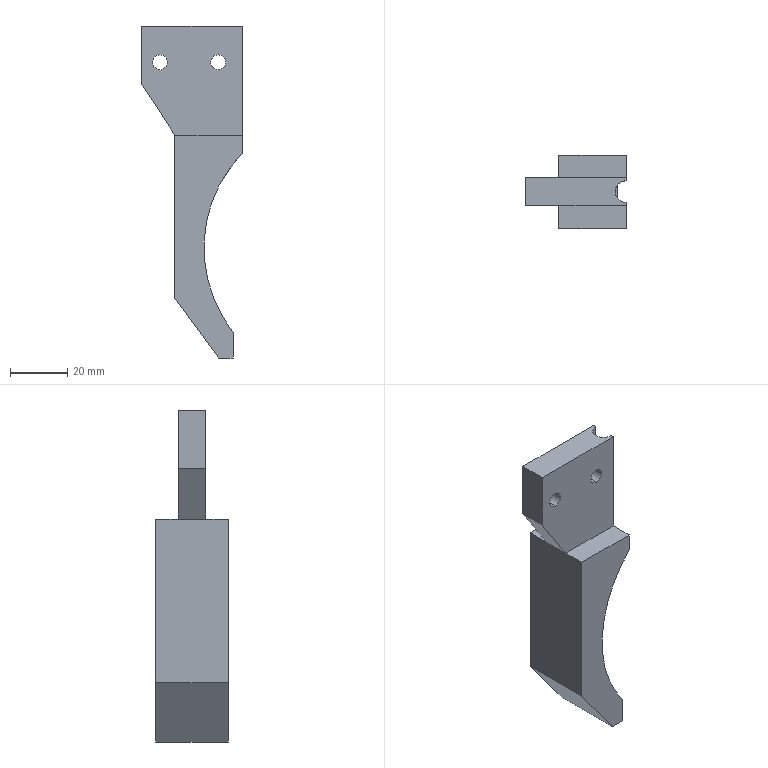Part | SolidWorks | features ICE 2, Extrusion 1 | 1 solid | 21 faces | box 35.052 x 25.4 x 115.945 mm | volume 36905 mm3 | plane 15 | cylinder 6 | commonest cylinder face diameters 5.207 x4 7.62 x1 95.25 x1
STEP:
#1=CARTESIAN_POINT('',(-8.382,4.826,62.197));
#2=VERTEX_POINT('',#1);
#3=CARTESIAN_POINT('',(-8.382,4.826,67.404));
#4=VERTEX_POINT('',#3);
#5=CARTESIAN_POINT('',(-8.382,4.826,64.801));
#6=DIRECTION('',(0.,1.,0.));
#7=DIRECTION('',(0.,0.,1.));
#8=AXIS2_PLACEMENT_3D('',#5,#6,#7);
#9=CIRCLE('',#8,2.603);
#10=EDGE_CURVE('',#2,#4,#9,.T.);
#11=ORIENTED_EDGE('',*,*,#10,.T.);
#12=CARTESIAN_POINT('',(-8.382,-4.826,67.404));
#13=VERTEX_POINT('',#12);
#14=CARTESIAN_POINT('',(-8.382,4.826,67.404));
#15=DIRECTION('',(0.,-1.,0.));
#16=VECTOR('',#15,1000.);
#17=LINE('',#14,#16);
#18=EDGE_CURVE('',#4,#13,#17,.T.);
#19=ORIENTED_EDGE('',*,*,#18,.T.);
#20=CARTESIAN_POINT('',(-8.382,-4.826,62.197));
#21=VERTEX_POINT('',#20);
#22=CARTESIAN_POINT('',(-8.382,-4.826,64.801));
#23=DIRECTION('',(0.,1.,0.));
#24=DIRECTION('',(0.,0.,1.));
#25=AXIS2_PLACEMENT_3D('',#22,#23,#24);
#26=CIRCLE('',#25,2.603);
#27=EDGE_CURVE('',#21,#13,#26,.T.);
#28=ORIENTED_EDGE('',*,*,#27,.F.);
#29=CARTESIAN_POINT('',(-8.382,4.826,62.197));
#30=DIRECTION('',(0.,-1.,0.));
#31=VECTOR('',#30,1000.);
#32=LINE('',#29,#31);
#33=EDGE_CURVE('',#2,#21,#32,.T.);
#34=ORIENTED_EDGE('',*,*,#33,.F.);
#35=EDGE_LOOP('',(#11,#19,#28,#34));
#36=FACE_OUTER_BOUND('',#35,.T.);
#37=CARTESIAN_POINT('',(-8.382,4.826,64.801));
#38=DIRECTION('',(0.,-1.,0.));
#39=DIRECTION('',(0.,0.,-1.));
#40=AXIS2_PLACEMENT_3D('',#37,#38,#39);
#41=CYLINDRICAL_SURFACE('',#40,2.603);
#42=ADVANCED_FACE('',(#36),#41,.F.);
#43=CARTESIAN_POINT('',(-28.702,4.826,62.197));
#44=VERTEX_POINT('',#43);
#45=CARTESIAN_POINT('',(-28.702,4.826,67.404));
#46=VERTEX_POINT('',#45);
#47=CARTESIAN_POINT('',(-28.702,4.826,64.801));
#48=DIRECTION('',(0.,1.,0.));
#49=DIRECTION('',(0.,0.,1.));
#50=AXIS2_PLACEMENT_3D('',#47,#48,#49);
#51=CIRCLE('',#50,2.603);
#52=EDGE_CURVE('',#44,#46,#51,.T.);
#53=ORIENTED_EDGE('',*,*,#52,.T.);
#54=CARTESIAN_POINT('',(-28.702,-4.826,67.404));
#55=VERTEX_POINT('',#54);
#56=CARTESIAN_POINT('',(-28.702,4.826,67.404));
#57=DIRECTION('',(0.,-1.,0.));
#58=VECTOR('',#57,1000.);
#59=LINE('',#56,#58);
#60=EDGE_CURVE('',#46,#55,#59,.T.);
#61=ORIENTED_EDGE('',*,*,#60,.T.);
#62=CARTESIAN_POINT('',(-28.702,-4.826,62.197));
#63=VERTEX_POINT('',#62);
#64=CARTESIAN_POINT('',(-28.702,-4.826,64.801));
#65=DIRECTION('',(0.,1.,0.));
#66=DIRECTION('',(0.,0.,1.));
#67=AXIS2_PLACEMENT_3D('',#64,#65,#66);
#68=CIRCLE('',#67,2.603);
#69=EDGE_CURVE('',#63,#55,#68,.T.);
#70=ORIENTED_EDGE('',*,*,#69,.F.);
#71=CARTESIAN_POINT('',(-28.702,4.826,62.197));
#72=DIRECTION('',(0.,-1.,0.));
#73=VECTOR('',#72,1000.);
#74=LINE('',#71,#73);
#75=EDGE_CURVE('',#44,#63,#74,.T.);
#76=ORIENTED_EDGE('',*,*,#75,.F.);
#77=EDGE_LOOP('',(#53,#61,#70,#76));
#78=FACE_OUTER_BOUND('',#77,.T.);
#79=CARTESIAN_POINT('',(-28.702,4.826,64.801));
#80=DIRECTION('',(0.,-1.,0.));
#81=DIRECTION('',(0.,0.,-1.));
#82=AXIS2_PLACEMENT_3D('',#79,#80,#81);
#83=CYLINDRICAL_SURFACE('',#82,2.604);
#84=ADVANCED_FACE('',(#78),#83,.F.);
#85=CARTESIAN_POINT('',(0.,3.81,33.051));
#86=VERTEX_POINT('',#85);
#87=CARTESIAN_POINT('',(0.,3.81,77.501));
#88=VERTEX_POINT('',#87);
#89=CARTESIAN_POINT('',(0.,3.81,27.463));
#90=DIRECTION('',(0.,0.,1.));
#91=VECTOR('',#90,1000.);
#92=LINE('',#89,#91);
#93=EDGE_CURVE('',#86,#88,#92,.T.);
#94=ORIENTED_EDGE('',*,*,#93,.F.);
#95=CARTESIAN_POINT('',(0.,12.7,33.051));
#96=VERTEX_POINT('',#95);
#97=CARTESIAN_POINT('',(0.,12.7,33.051));
#98=DIRECTION('',(0.,-1.,0.));
#99=VECTOR('',#98,1000.);
#100=LINE('',#97,#99);
#101=EDGE_CURVE('',#96,#86,#100,.T.);
#102=ORIENTED_EDGE('',*,*,#101,.F.);
#103=CARTESIAN_POINT('',(0.,12.7,39.401));
#104=VERTEX_POINT('',#103);
#105=CARTESIAN_POINT('',(0.,12.7,0.));
#106=DIRECTION('',(0.,0.,1.));
#107=VECTOR('',#106,1000.);
#108=LINE('',#105,#107);
#109=EDGE_CURVE('',#96,#104,#108,.T.);
#110=ORIENTED_EDGE('',*,*,#109,.T.);
#111=CARTESIAN_POINT('',(0.,4.826,39.401));
#112=VERTEX_POINT('',#111);
#113=CARTESIAN_POINT('',(0.,12.7,39.401));
#114=DIRECTION('',(0.,-1.,0.));
#115=VECTOR('',#114,1000.);
#116=LINE('',#113,#115);
#117=EDGE_CURVE('',#104,#112,#116,.T.);
#118=ORIENTED_EDGE('',*,*,#117,.T.);
#119=CARTESIAN_POINT('',(0.,4.826,77.501));
#120=VERTEX_POINT('',#119);
#121=CARTESIAN_POINT('',(0.,4.826,0.));
#122=DIRECTION('',(0.,0.,-1.));
#123=VECTOR('',#122,1000.);
#124=LINE('',#121,#123);
#125=EDGE_CURVE('',#120,#112,#124,.T.);
#126=ORIENTED_EDGE('',*,*,#125,.F.);
#127=CARTESIAN_POINT('',(0.,4.826,77.501));
#128=DIRECTION('',(0.,-1.,0.));
#129=VECTOR('',#128,1000.);
#130=LINE('',#127,#129);
#131=EDGE_CURVE('',#120,#88,#130,.T.);
#132=ORIENTED_EDGE('',*,*,#131,.T.);
#133=EDGE_LOOP('',(#94,#102,#110,#118,#126,#132));
#134=FACE_OUTER_BOUND('',#133,.T.);
#135=CARTESIAN_POINT('',(0.,12.7,0.));
#136=DIRECTION('',(1.,0.,0.));
#137=DIRECTION('',(0.,0.,-1.));
#138=AXIS2_PLACEMENT_3D('',#135,#136,#137);
#139=PLANE('',#138);
#140=ADVANCED_FACE('',(#134),#139,.T.);
#141=CARTESIAN_POINT('',(0.,-4.826,39.401));
#142=VERTEX_POINT('',#141);
#143=CARTESIAN_POINT('',(0.,-12.7,39.401));
#144=VERTEX_POINT('',#143);
#145=CARTESIAN_POINT('',(0.,12.7,39.401));
#146=DIRECTION('',(0.,-1.,0.));
#147=VECTOR('',#146,1000.);
#148=LINE('',#145,#147);
#149=EDGE_CURVE('',#142,#144,#148,.T.);
#150=ORIENTED_EDGE('',*,*,#149,.F.);
#151=CARTESIAN_POINT('',(-23.495,-4.826,39.401));
#152=VERTEX_POINT('',#151);
#153=CARTESIAN_POINT('',(0.,-4.826,39.401));
#154=DIRECTION('',(-1.,0.,0.));
#155=VECTOR('',#154,1000.);
#156=LINE('',#153,#155);
#157=EDGE_CURVE('',#142,#152,#156,.T.);
#158=ORIENTED_EDGE('',*,*,#157,.T.);
#159=CARTESIAN_POINT('',(-23.495,-12.7,39.401));
#160=VERTEX_POINT('',#159);
#161=CARTESIAN_POINT('',(-23.495,12.7,39.401));
#162=DIRECTION('',(0.,-1.,0.));
#163=VECTOR('',#162,1000.);
#164=LINE('',#161,#163);
#165=EDGE_CURVE('',#152,#160,#164,.T.);
#166=ORIENTED_EDGE('',*,*,#165,.T.);
#167=CARTESIAN_POINT('',(0.,-12.7,39.401));
#168=DIRECTION('',(-1.,0.,0.));
#169=VECTOR('',#168,1000.);
#170=LINE('',#167,#169);
#171=EDGE_CURVE('',#144,#160,#170,.T.);
#172=ORIENTED_EDGE('',*,*,#171,.F.);
#173=EDGE_LOOP('',(#150,#158,#166,#172));
#174=FACE_OUTER_BOUND('',#173,.T.);
#175=CARTESIAN_POINT('',(0.,12.7,39.401));
#176=DIRECTION('',(0.,0.,1.));
#177=DIRECTION('',(1.,0.,0.));
#178=AXIS2_PLACEMENT_3D('',#175,#176,#177);
#179=PLANE('',#178);
#180=ADVANCED_FACE('',(#174),#179,.T.);
#181=CARTESIAN_POINT('',(0.,-3.81,33.051));
#182=VERTEX_POINT('',#181);
#183=CARTESIAN_POINT('',(0.,-3.81,33.051));
#184=CARTESIAN_POINT('',(-0.4455,-3.81,32.588));
#185=CARTESIAN_POINT('',(-0.8726,-3.734,32.126));
#186=CARTESIAN_POINT('',(-1.488,-3.514,31.435));
#187=CARTESIAN_POINT('',(-1.69,-3.422,31.204));
#188=CARTESIAN_POINT('',(-2.08,-3.2,30.748));
#189=CARTESIAN_POINT('',(-2.268,-3.071,30.525));
#190=CARTESIAN_POINT('',(-2.625,-2.772,30.092));
#191=CARTESIAN_POINT('',(-2.795,-2.601,29.882));
#192=CARTESIAN_POINT('',(-3.113,-2.211,29.482));
#193=CARTESIAN_POINT('',(-3.258,-1.994,29.297));
#194=CARTESIAN_POINT('',(-3.448,-1.627,29.052));
#195=CARTESIAN_POINT('',(-3.507,-1.497,28.975));
#196=CARTESIAN_POINT('',(-3.61,-1.226,28.84));
#197=CARTESIAN_POINT('',(-3.655,-1.085,28.78));
#198=CARTESIAN_POINT('',(-3.73,-0.7896,28.681));
#199=CARTESIAN_POINT('',(-3.76,-0.6341,28.641));
#200=CARTESIAN_POINT('',(-3.8,-0.3211,28.589));
#201=CARTESIAN_POINT('',(-3.81,-0.1621,28.575));
#202=CARTESIAN_POINT('',(-3.81,0.1613,28.575));
#203=CARTESIAN_POINT('',(-3.8,0.3213,28.589));
#204=CARTESIAN_POINT('',(-3.76,0.6341,28.641));
#205=CARTESIAN_POINT('',(-3.731,0.789,28.681));
#206=CARTESIAN_POINT('',(-3.618,1.233,28.83));
#207=CARTESIAN_POINT('',(-3.512,1.503,28.969));
#208=CARTESIAN_POINT('',(-3.258,1.994,29.297));
#209=CARTESIAN_POINT('',(-3.114,2.21,29.482));
#210=CARTESIAN_POINT('',(-2.798,2.598,29.878));
#211=CARTESIAN_POINT('',(-2.626,2.77,30.09));
#212=CARTESIAN_POINT('',(-2.269,3.07,30.523));
#213=CARTESIAN_POINT('',(-2.083,3.198,30.745));
#214=CARTESIAN_POINT('',(-1.696,3.419,31.197));
#215=CARTESIAN_POINT('',(-1.494,3.512,31.429));
#216=CARTESIAN_POINT('',(-0.8737,3.734,32.125));
#217=CARTESIAN_POINT('',(-0.4451,3.81,32.589));
#218=CARTESIAN_POINT('',(0.,3.81,33.051));
#219=B_SPLINE_CURVE_WITH_KNOTS('',3,(#183,#184,#185,#186,#187,#188,#189,#190,#191,#192,#193,#194,#195,#196,#197,#198,#199,#200,#201,#202,#203,#204,#205,#206,#207,#208,#209,#210,#211,#212,#213,#214,#215,#216,#217,#218),.UNSPECIFIED.,.F.,.F.,(4,2,2,2,2,2,2,2,2,2,2,2,2,2,2,2,2,4),(0.,0.001898,0.002848,0.003797,0.004746,0.005695,0.00617,0.006645,0.007119,0.007594,0.008069,0.008543,0.009492,0.01044,0.01139,0.01234,0.01329,0.01519),.UNSPECIFIED.);
#220=EDGE_CURVE('',#182,#86,#219,.T.);
#221=ORIENTED_EDGE('',*,*,#220,.F.);
#222=CARTESIAN_POINT('',(0.,-12.7,33.051));
#223=VERTEX_POINT('',#222);
#224=CARTESIAN_POINT('',(0.,12.7,33.051));
#225=DIRECTION('',(0.,-1.,0.));
#226=VECTOR('',#225,1000.);
#227=LINE('',#224,#226);
#228=EDGE_CURVE('',#182,#223,#227,.T.);
#229=ORIENTED_EDGE('',*,*,#228,.T.);
#230=CARTESIAN_POINT('',(-3.175,-12.7,-29.403));
#231=VERTEX_POINT('',#230);
#232=CARTESIAN_POINT('',(34.29,-12.7,0.));
#233=DIRECTION('',(0.,1.,0.));
#234=DIRECTION('',(0.,0.,1.));
#235=AXIS2_PLACEMENT_3D('',#232,#233,#234);
#236=CIRCLE('',#235,47.625);
#237=EDGE_CURVE('',#231,#223,#236,.T.);
#238=ORIENTED_EDGE('',*,*,#237,.F.);
#239=CARTESIAN_POINT('',(-3.175,12.7,-29.403));
#240=VERTEX_POINT('',#239);
#241=CARTESIAN_POINT('',(-3.175,12.7,-29.403));
#242=DIRECTION('',(0.,-1.,0.));
#243=VECTOR('',#242,1000.);
#244=LINE('',#241,#243);
#245=EDGE_CURVE('',#240,#231,#244,.T.);
#246=ORIENTED_EDGE('',*,*,#245,.F.);
#247=CARTESIAN_POINT('',(34.29,12.7,0.));
#248=DIRECTION('',(0.,1.,0.));
#249=DIRECTION('',(0.,0.,1.));
#250=AXIS2_PLACEMENT_3D('',#247,#248,#249);
#251=CIRCLE('',#250,47.625);
#252=EDGE_CURVE('',#240,#96,#251,.T.);
#253=ORIENTED_EDGE('',*,*,#252,.T.);
#254=ORIENTED_EDGE('',*,*,#101,.T.);
#255=EDGE_LOOP('',(#221,#229,#238,#246,#253,#254));
#256=FACE_OUTER_BOUND('',#255,.T.);
#257=CARTESIAN_POINT('',(34.29,12.7,0.));
#258=DIRECTION('',(0.,-1.,0.));
#259=DIRECTION('',(0.,0.,-1.));
#260=AXIS2_PLACEMENT_3D('',#257,#258,#259);
#261=CYLINDRICAL_SURFACE('',#260,47.625);
#262=ADVANCED_FACE('',(#256),#261,.F.);
#263=CARTESIAN_POINT('',(-3.175,-12.7,-38.444));
#264=VERTEX_POINT('',#263);
#265=CARTESIAN_POINT('',(-3.175,-12.7,0.));
#266=DIRECTION('',(0.,0.,-1.));
#267=VECTOR('',#266,1000.);
#268=LINE('',#265,#267);
#269=EDGE_CURVE('',#231,#264,#268,.T.);
#270=ORIENTED_EDGE('',*,*,#269,.T.);
#271=CARTESIAN_POINT('',(-3.175,12.7,-38.444));
#272=VERTEX_POINT('',#271);
#273=CARTESIAN_POINT('',(-3.175,12.7,-38.444));
#274=DIRECTION('',(0.,-1.,0.));
#275=VECTOR('',#274,1000.);
#276=LINE('',#273,#275);
#277=EDGE_CURVE('',#272,#264,#276,.T.);
#278=ORIENTED_EDGE('',*,*,#277,.F.);
#279=CARTESIAN_POINT('',(-3.175,12.7,0.));
#280=DIRECTION('',(0.,0.,-1.));
#281=VECTOR('',#280,1000.);
#282=LINE('',#279,#281);
#283=EDGE_CURVE('',#240,#272,#282,.T.);
#284=ORIENTED_EDGE('',*,*,#283,.F.);
#285=ORIENTED_EDGE('',*,*,#245,.T.);
#286=EDGE_LOOP('',(#270,#278,#284,#285));
#287=FACE_OUTER_BOUND('',#286,.T.);
#288=CARTESIAN_POINT('',(-3.175,12.7,0.));
#289=DIRECTION('',(-1.,0.,0.));
#290=DIRECTION('',(0.,0.,1.));
#291=AXIS2_PLACEMENT_3D('',#288,#289,#290);
#292=PLANE('',#291);
#293=ADVANCED_FACE('',(#287),#292,.F.);
#294=CARTESIAN_POINT('',(-8.255,-12.7,-38.444));
#295=VERTEX_POINT('',#294);
#296=CARTESIAN_POINT('',(0.,-12.7,-38.444));
#297=DIRECTION('',(1.,0.,0.));
#298=VECTOR('',#297,1000.);
#299=LINE('',#296,#298);
#300=EDGE_CURVE('',#295,#264,#299,.T.);
#301=ORIENTED_EDGE('',*,*,#300,.F.);
#302=CARTESIAN_POINT('',(-8.255,12.7,-38.444));
#303=VERTEX_POINT('',#302);
#304=CARTESIAN_POINT('',(-8.255,12.7,-38.444));
#305=DIRECTION('',(0.,-1.,0.));
#306=VECTOR('',#305,1000.);
#307=LINE('',#304,#306);
#308=EDGE_CURVE('',#303,#295,#307,.T.);
#309=ORIENTED_EDGE('',*,*,#308,.F.);
#310=CARTESIAN_POINT('',(0.,12.7,-38.444));
#311=DIRECTION('',(1.,0.,0.));
#312=VECTOR('',#311,1000.);
#313=LINE('',#310,#312);
#314=EDGE_CURVE('',#303,#272,#313,.T.);
#315=ORIENTED_EDGE('',*,*,#314,.T.);
#316=ORIENTED_EDGE('',*,*,#277,.T.);
#317=EDGE_LOOP('',(#301,#309,#315,#316));
#318=FACE_OUTER_BOUND('',#317,.T.);
#319=CARTESIAN_POINT('',(0.,12.7,-38.444));
#320=DIRECTION('',(0.,0.,-1.));
#321=DIRECTION('',(-1.,0.,0.));
#322=AXIS2_PLACEMENT_3D('',#319,#320,#321);
#323=PLANE('',#322);
#324=ADVANCED_FACE('',(#318),#323,.T.);
#325=CARTESIAN_POINT('',(-23.495,-12.7,-17.749));
#326=VERTEX_POINT('',#325);
#327=CARTESIAN_POINT('',(-23.709,-12.7,-17.459));
#328=DIRECTION('',(0.593,0.,-0.8052));
#329=VECTOR('',#328,1000.);
#330=LINE('',#327,#329);
#331=EDGE_CURVE('',#326,#295,#330,.T.);
#332=ORIENTED_EDGE('',*,*,#331,.F.);
#333=CARTESIAN_POINT('',(-23.495,12.7,-17.749));
#334=VERTEX_POINT('',#333);
#335=CARTESIAN_POINT('',(-23.495,12.7,-17.749));
#336=DIRECTION('',(0.,-1.,0.));
#337=VECTOR('',#336,1000.);
#338=LINE('',#335,#337);
#339=EDGE_CURVE('',#334,#326,#338,.T.);
#340=ORIENTED_EDGE('',*,*,#339,.F.);
#341=CARTESIAN_POINT('',(-23.709,12.7,-17.459));
#342=DIRECTION('',(0.593,0.,-0.8052));
#343=VECTOR('',#342,1000.);
#344=LINE('',#341,#343);
#345=EDGE_CURVE('',#334,#303,#344,.T.);
#346=ORIENTED_EDGE('',*,*,#345,.T.);
#347=ORIENTED_EDGE('',*,*,#308,.T.);
#348=EDGE_LOOP('',(#332,#340,#346,#347));
#349=FACE_OUTER_BOUND('',#348,.T.);
#350=CARTESIAN_POINT('',(-23.709,12.7,-17.459));
#351=DIRECTION('',(-0.8052,0.,-0.593));
#352=DIRECTION('',(-0.593,0.,0.8052));
#353=AXIS2_PLACEMENT_3D('',#350,#351,#352);
#354=PLANE('',#353);
#355=ADVANCED_FACE('',(#349),#354,.T.);
#356=CARTESIAN_POINT('',(-23.495,-12.7,0.));
#357=DIRECTION('',(0.,0.,1.));
#358=VECTOR('',#357,1000.);
#359=LINE('',#356,#358);
#360=EDGE_CURVE('',#326,#160,#359,.T.);
#361=ORIENTED_EDGE('',*,*,#360,.T.);
#362=ORIENTED_EDGE('',*,*,#165,.F.);
#363=CARTESIAN_POINT('',(-23.495,4.826,39.401));
#364=VERTEX_POINT('',#363);
#365=CARTESIAN_POINT('',(-23.495,4.826,39.401));
#366=DIRECTION('',(0.,-1.,0.));
#367=VECTOR('',#366,1000.);
#368=LINE('',#365,#367);
#369=EDGE_CURVE('',#364,#152,#368,.T.);
#370=ORIENTED_EDGE('',*,*,#369,.F.);
#371=CARTESIAN_POINT('',(-23.495,12.7,39.401));
#372=VERTEX_POINT('',#371);
#373=CARTESIAN_POINT('',(-23.495,12.7,39.401));
#374=DIRECTION('',(0.,-1.,0.));
#375=VECTOR('',#374,1000.);
#376=LINE('',#373,#375);
#377=EDGE_CURVE('',#372,#364,#376,.T.);
#378=ORIENTED_EDGE('',*,*,#377,.F.);
#379=CARTESIAN_POINT('',(-23.495,12.7,0.));
#380=DIRECTION('',(0.,0.,1.));
#381=VECTOR('',#380,1000.);
#382=LINE('',#379,#381);
#383=EDGE_CURVE('',#334,#372,#382,.T.);
#384=ORIENTED_EDGE('',*,*,#383,.F.);
#385=ORIENTED_EDGE('',*,*,#339,.T.);
#386=EDGE_LOOP('',(#361,#362,#370,#378,#384,#385));
#387=FACE_OUTER_BOUND('',#386,.T.);
#388=CARTESIAN_POINT('',(-23.495,12.7,0.));
#389=DIRECTION('',(1.,0.,0.));
#390=DIRECTION('',(0.,0.,-1.));
#391=AXIS2_PLACEMENT_3D('',#388,#389,#390);
#392=PLANE('',#391);
#393=ADVANCED_FACE('',(#387),#392,.F.);
#394=CARTESIAN_POINT('',(0.,4.826,39.401));
#395=DIRECTION('',(-1.,0.,0.));
#396=VECTOR('',#395,1000.);
#397=LINE('',#394,#396);
#398=EDGE_CURVE('',#112,#364,#397,.T.);
#399=ORIENTED_EDGE('',*,*,#398,.F.);
#400=ORIENTED_EDGE('',*,*,#117,.F.);
#401=CARTESIAN_POINT('',(0.,12.7,39.401));
#402=DIRECTION('',(-1.,0.,0.));
#403=VECTOR('',#402,1000.);
#404=LINE('',#401,#403);
#405=EDGE_CURVE('',#104,#372,#404,.T.);
#406=ORIENTED_EDGE('',*,*,#405,.T.);
#407=ORIENTED_EDGE('',*,*,#377,.T.);
#408=EDGE_LOOP('',(#399,#400,#406,#407));
#409=FACE_OUTER_BOUND('',#408,.T.);
#410=CARTESIAN_POINT('',(0.,12.7,39.401));
#411=DIRECTION('',(0.,0.,1.));
#412=DIRECTION('',(1.,0.,0.));
#413=AXIS2_PLACEMENT_3D('',#410,#411,#412);
#414=PLANE('',#413);
#415=ADVANCED_FACE('',(#409),#414,.T.);
#416=CARTESIAN_POINT('',(0.,-3.81,77.501));
#417=VERTEX_POINT('',#416);
#418=CARTESIAN_POINT('',(0.,-3.81,27.463));
#419=DIRECTION('',(0.,0.,-1.));
#420=VECTOR('',#419,1000.);
#421=LINE('',#418,#420);
#422=EDGE_CURVE('',#417,#182,#421,.T.);
#423=ORIENTED_EDGE('',*,*,#422,.F.);
#424=CARTESIAN_POINT('',(0.,-4.826,77.501));
#425=VERTEX_POINT('',#424);
#426=CARTESIAN_POINT('',(0.,4.826,77.501));
#427=DIRECTION('',(0.,-1.,0.));
#428=VECTOR('',#427,1000.);
#429=LINE('',#426,#428);
#430=EDGE_CURVE('',#417,#425,#429,.T.);
#431=ORIENTED_EDGE('',*,*,#430,.T.);
#432=CARTESIAN_POINT('',(0.,-4.826,0.));
#433=DIRECTION('',(0.,0.,-1.));
#434=VECTOR('',#433,1000.);
#435=LINE('',#432,#434);
#436=EDGE_CURVE('',#425,#142,#435,.T.);
#437=ORIENTED_EDGE('',*,*,#436,.T.);
#438=ORIENTED_EDGE('',*,*,#149,.T.);
#439=CARTESIAN_POINT('',(0.,-12.7,0.));
#440=DIRECTION('',(0.,0.,1.));
#441=VECTOR('',#440,1000.);
#442=LINE('',#439,#441);
#443=EDGE_CURVE('',#223,#144,#442,.T.);
#444=ORIENTED_EDGE('',*,*,#443,.F.);
#445=ORIENTED_EDGE('',*,*,#228,.F.);
#446=EDGE_LOOP('',(#423,#431,#437,#438,#444,#445));
#447=FACE_OUTER_BOUND('',#446,.T.);
#448=CARTESIAN_POINT('',(0.,12.7,0.));
#449=DIRECTION('',(1.,0.,0.));
#450=DIRECTION('',(0.,0.,-1.));
#451=AXIS2_PLACEMENT_3D('',#448,#449,#450);
#452=PLANE('',#451);
#453=ADVANCED_FACE('',(#447),#452,.T.);
#454=ORIENTED_EDGE('',*,*,#252,.F.);
#455=ORIENTED_EDGE('',*,*,#283,.T.);
#456=ORIENTED_EDGE('',*,*,#314,.F.);
#457=ORIENTED_EDGE('',*,*,#345,.F.);
#458=ORIENTED_EDGE('',*,*,#383,.T.);
#459=ORIENTED_EDGE('',*,*,#405,.F.);
#460=ORIENTED_EDGE('',*,*,#109,.F.);
#461=EDGE_LOOP('',(#454,#455,#456,#457,#458,#459,#460));
#462=FACE_OUTER_BOUND('',#461,.T.);
#463=CARTESIAN_POINT('',(0.,12.7,0.));
#464=DIRECTION('',(0.,1.,0.));
#465=DIRECTION('',(0.,0.,1.));
#466=AXIS2_PLACEMENT_3D('',#463,#464,#465);
#467=PLANE('',#466);
#468=ADVANCED_FACE('',(#462),#467,.T.);
#469=ORIENTED_EDGE('',*,*,#237,.T.);
#470=ORIENTED_EDGE('',*,*,#443,.T.);
#471=ORIENTED_EDGE('',*,*,#171,.T.);
#472=ORIENTED_EDGE('',*,*,#360,.F.);
#473=ORIENTED_EDGE('',*,*,#331,.T.);
#474=ORIENTED_EDGE('',*,*,#300,.T.);
#475=ORIENTED_EDGE('',*,*,#269,.F.);
#476=EDGE_LOOP('',(#469,#470,#471,#472,#473,#474,#475));
#477=FACE_OUTER_BOUND('',#476,.T.);
#478=CARTESIAN_POINT('',(0.,-12.7,0.));
#479=DIRECTION('',(0.,1.,0.));
#480=DIRECTION('',(0.,0.,1.));
#481=AXIS2_PLACEMENT_3D('',#478,#479,#480);
#482=PLANE('',#481);
#483=ADVANCED_FACE('',(#477),#482,.F.);
#484=ORIENTED_EDGE('',*,*,#430,.F.);
#485=CARTESIAN_POINT('',(0.,0.,77.501));
#486=DIRECTION('',(0.,0.,1.));
#487=DIRECTION('',(1.,0.,0.));
#488=AXIS2_PLACEMENT_3D('',#485,#486,#487);
#489=CIRCLE('',#488,3.81);
#490=EDGE_CURVE('',#88,#417,#489,.T.);
#491=ORIENTED_EDGE('',*,*,#490,.F.);
#492=ORIENTED_EDGE('',*,*,#131,.F.);
#493=CARTESIAN_POINT('',(-35.052,4.826,77.501));
#494=VERTEX_POINT('',#493);
#495=CARTESIAN_POINT('',(0.,4.826,77.501));
#496=DIRECTION('',(1.,0.,0.));
#497=VECTOR('',#496,1000.);
#498=LINE('',#495,#497);
#499=EDGE_CURVE('',#494,#120,#498,.T.);
#500=ORIENTED_EDGE('',*,*,#499,.F.);
#501=CARTESIAN_POINT('',(-35.052,-4.826,77.501));
#502=VERTEX_POINT('',#501);
#503=CARTESIAN_POINT('',(-35.052,4.826,77.501));
#504=DIRECTION('',(0.,-1.,0.));
#505=VECTOR('',#504,1000.);
#506=LINE('',#503,#505);
#507=EDGE_CURVE('',#494,#502,#506,.T.);
#508=ORIENTED_EDGE('',*,*,#507,.T.);
#509=CARTESIAN_POINT('',(0.,-4.826,77.501));
#510=DIRECTION('',(1.,0.,0.));
#511=VECTOR('',#510,1000.);
#512=LINE('',#509,#511);
#513=EDGE_CURVE('',#502,#425,#512,.T.);
#514=ORIENTED_EDGE('',*,*,#513,.T.);
#515=EDGE_LOOP('',(#484,#491,#492,#500,#508,#514));
#516=FACE_OUTER_BOUND('',#515,.T.);
#517=CARTESIAN_POINT('',(0.,4.826,77.501));
#518=DIRECTION('',(0.,0.,-1.));
#519=DIRECTION('',(-1.,0.,0.));
#520=AXIS2_PLACEMENT_3D('',#517,#518,#519);
#521=PLANE('',#520);
#522=ADVANCED_FACE('',(#516),#521,.F.);
#523=CARTESIAN_POINT('',(-35.052,-4.826,57.181));
#524=VERTEX_POINT('',#523);
#525=CARTESIAN_POINT('',(1.487,-4.826,0.9666));
#526=DIRECTION('',(-0.545,0.,0.8384));
#527=VECTOR('',#526,1000.);
#528=LINE('',#525,#527);
#529=EDGE_CURVE('',#152,#524,#528,.T.);
#530=ORIENTED_EDGE('',*,*,#529,.T.);
#531=CARTESIAN_POINT('',(-35.052,4.826,57.181));
#532=VERTEX_POINT('',#531);
#533=CARTESIAN_POINT('',(-35.052,4.826,57.181));
#534=DIRECTION('',(0.,-1.,0.));
#535=VECTOR('',#534,1000.);
#536=LINE('',#533,#535);
#537=EDGE_CURVE('',#532,#524,#536,.T.);
#538=ORIENTED_EDGE('',*,*,#537,.F.);
#539=CARTESIAN_POINT('',(1.487,4.826,0.9666));
#540=DIRECTION('',(-0.545,0.,0.8384));
#541=VECTOR('',#540,1000.);
#542=LINE('',#539,#541);
#543=EDGE_CURVE('',#364,#532,#542,.T.);
#544=ORIENTED_EDGE('',*,*,#543,.F.);
#545=ORIENTED_EDGE('',*,*,#369,.T.);
#546=EDGE_LOOP('',(#530,#538,#544,#545));
#547=FACE_OUTER_BOUND('',#546,.T.);
#548=CARTESIAN_POINT('',(1.487,4.826,0.9666));
#549=DIRECTION('',(0.8384,0.,0.545));
#550=DIRECTION('',(0.545,0.,-0.8384));
#551=AXIS2_PLACEMENT_3D('',#548,#549,#550);
#552=PLANE('',#551);
#553=ADVANCED_FACE('',(#547),#552,.F.);
#554=ORIENTED_EDGE('',*,*,#60,.F.);
#555=CARTESIAN_POINT('',(-28.702,4.826,64.801));
#556=DIRECTION('',(0.,1.,0.));
#557=DIRECTION('',(0.,0.,1.));
#558=AXIS2_PLACEMENT_3D('',#555,#556,#557);
#559=CIRCLE('',#558,2.603);
#560=EDGE_CURVE('',#46,#44,#559,.T.);
#561=ORIENTED_EDGE('',*,*,#560,.T.);
#562=ORIENTED_EDGE('',*,*,#75,.T.);
#563=CARTESIAN_POINT('',(-28.702,-4.826,64.801));
#564=DIRECTION('',(0.,1.,0.));
#565=DIRECTION('',(0.,0.,1.));
#566=AXIS2_PLACEMENT_3D('',#563,#564,#565);
#567=CIRCLE('',#566,2.603);
#568=EDGE_CURVE('',#55,#63,#567,.T.);
#569=ORIENTED_EDGE('',*,*,#568,.F.);
#570=EDGE_LOOP('',(#554,#561,#562,#569));
#571=FACE_OUTER_BOUND('',#570,.T.);
#572=CARTESIAN_POINT('',(-28.702,4.826,64.801));
#573=DIRECTION('',(0.,-1.,0.));
#574=DIRECTION('',(0.,0.,-1.));
#575=AXIS2_PLACEMENT_3D('',#572,#573,#574);
#576=CYLINDRICAL_SURFACE('',#575,2.604);
#577=ADVANCED_FACE('',(#571),#576,.F.);
#578=ORIENTED_EDGE('',*,*,#18,.F.);
#579=CARTESIAN_POINT('',(-8.382,4.826,64.801));
#580=DIRECTION('',(0.,1.,0.));
#581=DIRECTION('',(0.,0.,1.));
#582=AXIS2_PLACEMENT_3D('',#579,#580,#581);
#583=CIRCLE('',#582,2.603);
#584=EDGE_CURVE('',#4,#2,#583,.T.);
#585=ORIENTED_EDGE('',*,*,#584,.T.);
#586=ORIENTED_EDGE('',*,*,#33,.T.);
#587=CARTESIAN_POINT('',(-8.382,-4.826,64.801));
#588=DIRECTION('',(0.,1.,0.));
#589=DIRECTION('',(0.,0.,1.));
#590=AXIS2_PLACEMENT_3D('',#587,#588,#589);
#591=CIRCLE('',#590,2.603);
#592=EDGE_CURVE('',#13,#21,#591,.T.);
#593=ORIENTED_EDGE('',*,*,#592,.F.);
#594=EDGE_LOOP('',(#578,#585,#586,#593));
#595=FACE_OUTER_BOUND('',#594,.T.);
#596=CARTESIAN_POINT('',(-8.382,4.826,64.801));
#597=DIRECTION('',(0.,-1.,0.));
#598=DIRECTION('',(0.,0.,-1.));
#599=AXIS2_PLACEMENT_3D('',#596,#597,#598);
#600=CYLINDRICAL_SURFACE('',#599,2.603);
#601=ADVANCED_FACE('',(#595),#600,.F.);
#602=CARTESIAN_POINT('',(-35.052,-4.826,0.));
#603=DIRECTION('',(0.,0.,1.));
#604=VECTOR('',#603,1000.);
#605=LINE('',#602,#604);
#606=EDGE_CURVE('',#524,#502,#605,.T.);
#607=ORIENTED_EDGE('',*,*,#606,.T.);
#608=ORIENTED_EDGE('',*,*,#507,.F.);
#609=CARTESIAN_POINT('',(-35.052,4.826,0.));
#610=DIRECTION('',(0.,0.,1.));
#611=VECTOR('',#610,1000.);
#612=LINE('',#609,#611);
#613=EDGE_CURVE('',#532,#494,#612,.T.);
#614=ORIENTED_EDGE('',*,*,#613,.F.);
#615=ORIENTED_EDGE('',*,*,#537,.T.);
#616=EDGE_LOOP('',(#607,#608,#614,#615));
#617=FACE_OUTER_BOUND('',#616,.T.);
#618=CARTESIAN_POINT('',(-35.052,4.826,0.));
#619=DIRECTION('',(1.,0.,0.));
#620=DIRECTION('',(0.,0.,-1.));
#621=AXIS2_PLACEMENT_3D('',#618,#619,#620);
#622=PLANE('',#621);
#623=ADVANCED_FACE('',(#617),#622,.F.);
#624=ORIENTED_EDGE('',*,*,#10,.F.);
#625=ORIENTED_EDGE('',*,*,#584,.F.);
#626=EDGE_LOOP('',(#624,#625));
#627=FACE_BOUND('',#626,.T.);
#628=ORIENTED_EDGE('',*,*,#52,.F.);
#629=ORIENTED_EDGE('',*,*,#560,.F.);
#630=EDGE_LOOP('',(#628,#629));
#631=FACE_BOUND('',#630,.T.);
#632=ORIENTED_EDGE('',*,*,#499,.T.);
#633=ORIENTED_EDGE('',*,*,#125,.T.);
#634=ORIENTED_EDGE('',*,*,#398,.T.);
#635=ORIENTED_EDGE('',*,*,#543,.T.);
#636=ORIENTED_EDGE('',*,*,#613,.T.);
#637=EDGE_LOOP('',(#632,#633,#634,#635,#636));
#638=FACE_OUTER_BOUND('',#637,.T.);
#639=CARTESIAN_POINT('',(0.,4.826,0.));
#640=DIRECTION('',(0.,1.,0.));
#641=DIRECTION('',(0.,0.,1.));
#642=AXIS2_PLACEMENT_3D('',#639,#640,#641);
#643=PLANE('',#642);
#644=ADVANCED_FACE('',(#627,#631,#638),#643,.T.);
#645=ORIENTED_EDGE('',*,*,#27,.T.);
#646=ORIENTED_EDGE('',*,*,#592,.T.);
#647=EDGE_LOOP('',(#645,#646));
#648=FACE_BOUND('',#647,.T.);
#649=ORIENTED_EDGE('',*,*,#69,.T.);
#650=ORIENTED_EDGE('',*,*,#568,.T.);
#651=EDGE_LOOP('',(#649,#650));
#652=FACE_BOUND('',#651,.T.);
#653=ORIENTED_EDGE('',*,*,#513,.F.);
#654=ORIENTED_EDGE('',*,*,#606,.F.);
#655=ORIENTED_EDGE('',*,*,#529,.F.);
#656=ORIENTED_EDGE('',*,*,#157,.F.);
#657=ORIENTED_EDGE('',*,*,#436,.F.);
#658=EDGE_LOOP('',(#653,#654,#655,#656,#657));
#659=FACE_OUTER_BOUND('',#658,.T.);
#660=CARTESIAN_POINT('',(0.,-4.826,0.));
#661=DIRECTION('',(0.,1.,0.));
#662=DIRECTION('',(0.,0.,1.));
#663=AXIS2_PLACEMENT_3D('',#660,#661,#662);
#664=PLANE('',#663);
#665=ADVANCED_FACE('',(#648,#652,#659),#664,.F.);
#666=ORIENTED_EDGE('',*,*,#93,.T.);
#667=ORIENTED_EDGE('',*,*,#490,.T.);
#668=ORIENTED_EDGE('',*,*,#422,.T.);
#669=ORIENTED_EDGE('',*,*,#220,.T.);
#670=EDGE_LOOP('',(#666,#667,#668,#669));
#671=FACE_OUTER_BOUND('',#670,.T.);
#672=CARTESIAN_POINT('',(0.,0.,27.463));
#673=DIRECTION('',(0.,0.,1.));
#674=DIRECTION('',(1.,0.,0.));
#675=AXIS2_PLACEMENT_3D('',#672,#673,#674);
#676=CYLINDRICAL_SURFACE('',#675,3.81);
#677=ADVANCED_FACE('',(#671),#676,.F.);
#678=CLOSED_SHELL('',(#42,#84,#140,#180,#262,#293,#324,#355,#393,#415,#453,#468,#483,#522,#553,#577,#601,#623,#644,#665,#677));
#679=MANIFOLD_SOLID_BREP('',#678);
#680=CARTESIAN_POINT('',(0.,0.,0.));
#681=DIRECTION('',(0.,0.,1.));
#682=DIRECTION('',(1.,0.,0.));
#683=AXIS2_PLACEMENT_3D('',#680,#681,#682);
#684=(LENGTH_UNIT()NAMED_UNIT(*)SI_UNIT(.MILLI.,.METRE.));
#685=UNCERTAINTY_MEASURE_WITH_UNIT(LENGTH_MEASURE(0.00001),#684,'','');
#686=(NAMED_UNIT(*)PLANE_ANGLE_UNIT()SI_UNIT($,.RADIAN.));
#687=(NAMED_UNIT(*)SI_UNIT($,.STERADIAN.)SOLID_ANGLE_UNIT());
#688=(GEOMETRIC_REPRESENTATION_CONTEXT(3)GLOBAL_UNCERTAINTY_ASSIGNED_CONTEXT((#685))GLOBAL_UNIT_ASSIGNED_CONTEXT((#684,#686,#687))REPRESENTATION_CONTEXT('',''));
#689=ADVANCED_BREP_SHAPE_REPRESENTATION('',(#679,#683),#688);